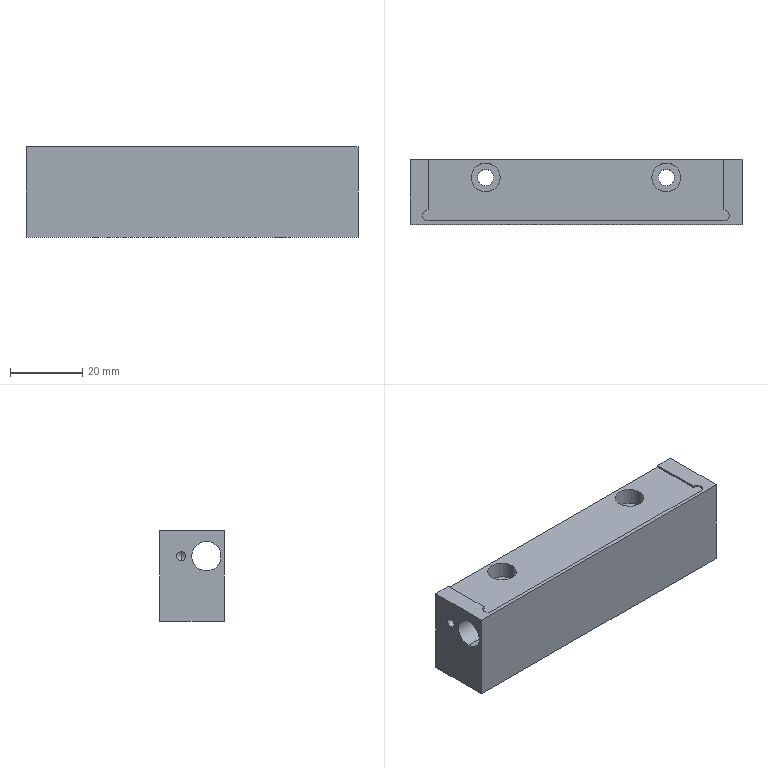Part | STEP file | 2063 Heat press block A | 1 solid | 40 faces | box 92 x 18 x 25 mm | volume 33821 mm3 | cylinder 21 | plane 13 | cone 6 | commonest cylinder face diameters 2.5 x4 4.5 x4 8 x4 3 x3 4.9 x2 5 x2